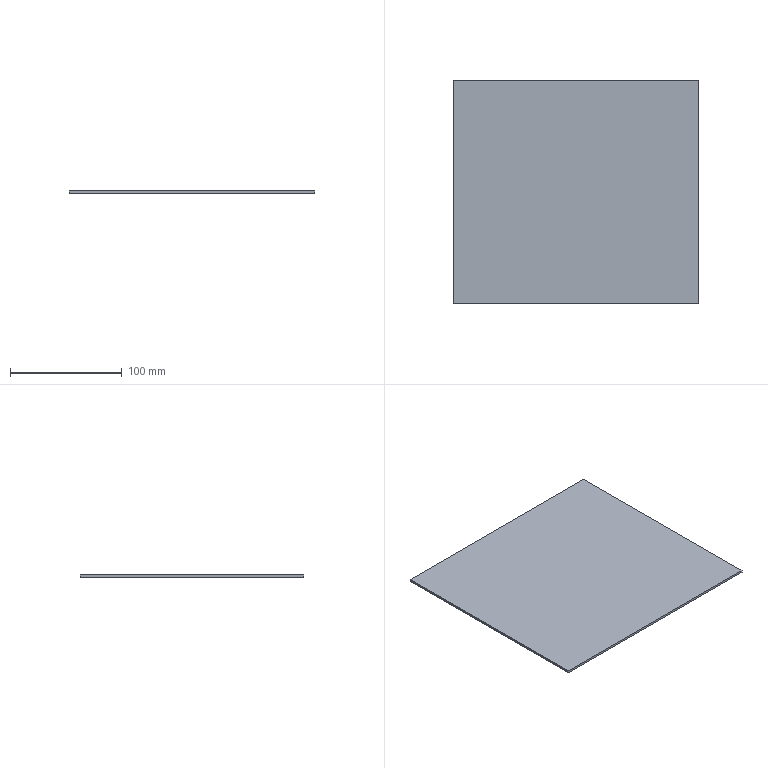Part | SolidWorks | features Extrusion 1 | 1 solid | 6 faces | box 220 x 200 x 2 mm | volume 88000 mm3 | plane 6
STEP:
#1=CARTESIAN_POINT('',(96.32,-91.,0.));
#2=VERTEX_POINT('',#1);
#3=CARTESIAN_POINT('',(96.32,109.,0.));
#4=VERTEX_POINT('',#3);
#5=CARTESIAN_POINT('',(96.32,-91.,0.));
#6=DIRECTION('',(0.,1.,0.));
#7=VECTOR('',#6,1000.);
#8=LINE('',#5,#7);
#9=EDGE_CURVE('',#2,#4,#8,.T.);
#10=ORIENTED_EDGE('',*,*,#9,.T.);
#11=CARTESIAN_POINT('',(96.32,109.,2.));
#12=VERTEX_POINT('',#11);
#13=CARTESIAN_POINT('',(96.32,109.,2.));
#14=DIRECTION('',(0.,0.,-1.));
#15=VECTOR('',#14,1000.);
#16=LINE('',#13,#15);
#17=EDGE_CURVE('',#12,#4,#16,.T.);
#18=ORIENTED_EDGE('',*,*,#17,.F.);
#19=CARTESIAN_POINT('',(96.32,-91.,2.));
#20=VERTEX_POINT('',#19);
#21=CARTESIAN_POINT('',(96.32,-91.,2.));
#22=DIRECTION('',(0.,1.,0.));
#23=VECTOR('',#22,1000.);
#24=LINE('',#21,#23);
#25=EDGE_CURVE('',#20,#12,#24,.T.);
#26=ORIENTED_EDGE('',*,*,#25,.F.);
#27=CARTESIAN_POINT('',(96.32,-91.,2.));
#28=DIRECTION('',(0.,0.,-1.));
#29=VECTOR('',#28,1000.);
#30=LINE('',#27,#29);
#31=EDGE_CURVE('',#20,#2,#30,.T.);
#32=ORIENTED_EDGE('',*,*,#31,.T.);
#33=EDGE_LOOP('',(#10,#18,#26,#32));
#34=FACE_OUTER_BOUND('',#33,.T.);
#35=CARTESIAN_POINT('',(96.32,-91.,2.));
#36=DIRECTION('',(-1.,0.,0.));
#37=DIRECTION('',(0.,0.,1.));
#38=AXIS2_PLACEMENT_3D('',#35,#36,#37);
#39=PLANE('',#38);
#40=ADVANCED_FACE('',(#34),#39,.F.);
#41=CARTESIAN_POINT('',(-123.68,109.,0.));
#42=VERTEX_POINT('',#41);
#43=CARTESIAN_POINT('',(96.32,109.,0.));
#44=DIRECTION('',(-1.,0.,0.));
#45=VECTOR('',#44,1000.);
#46=LINE('',#43,#45);
#47=EDGE_CURVE('',#4,#42,#46,.T.);
#48=ORIENTED_EDGE('',*,*,#47,.T.);
#49=CARTESIAN_POINT('',(-123.68,109.,2.));
#50=VERTEX_POINT('',#49);
#51=CARTESIAN_POINT('',(-123.68,109.,2.));
#52=DIRECTION('',(0.,0.,-1.));
#53=VECTOR('',#52,1000.);
#54=LINE('',#51,#53);
#55=EDGE_CURVE('',#50,#42,#54,.T.);
#56=ORIENTED_EDGE('',*,*,#55,.F.);
#57=CARTESIAN_POINT('',(96.32,109.,2.));
#58=DIRECTION('',(-1.,0.,0.));
#59=VECTOR('',#58,1000.);
#60=LINE('',#57,#59);
#61=EDGE_CURVE('',#12,#50,#60,.T.);
#62=ORIENTED_EDGE('',*,*,#61,.F.);
#63=ORIENTED_EDGE('',*,*,#17,.T.);
#64=EDGE_LOOP('',(#48,#56,#62,#63));
#65=FACE_OUTER_BOUND('',#64,.T.);
#66=CARTESIAN_POINT('',(96.32,109.,2.));
#67=DIRECTION('',(0.,-1.,0.));
#68=DIRECTION('',(1.,0.,0.));
#69=AXIS2_PLACEMENT_3D('',#66,#67,#68);
#70=PLANE('',#69);
#71=ADVANCED_FACE('',(#65),#70,.F.);
#72=CARTESIAN_POINT('',(-123.68,-91.,0.));
#73=VERTEX_POINT('',#72);
#74=CARTESIAN_POINT('',(-123.68,-91.,0.));
#75=DIRECTION('',(0.,1.,0.));
#76=VECTOR('',#75,1000.);
#77=LINE('',#74,#76);
#78=EDGE_CURVE('',#73,#42,#77,.T.);
#79=ORIENTED_EDGE('',*,*,#78,.F.);
#80=CARTESIAN_POINT('',(-123.68,-91.,2.));
#81=VERTEX_POINT('',#80);
#82=CARTESIAN_POINT('',(-123.68,-91.,2.));
#83=DIRECTION('',(0.,0.,-1.));
#84=VECTOR('',#83,1000.);
#85=LINE('',#82,#84);
#86=EDGE_CURVE('',#81,#73,#85,.T.);
#87=ORIENTED_EDGE('',*,*,#86,.F.);
#88=CARTESIAN_POINT('',(-123.68,-91.,2.));
#89=DIRECTION('',(0.,1.,0.));
#90=VECTOR('',#89,1000.);
#91=LINE('',#88,#90);
#92=EDGE_CURVE('',#81,#50,#91,.T.);
#93=ORIENTED_EDGE('',*,*,#92,.T.);
#94=ORIENTED_EDGE('',*,*,#55,.T.);
#95=EDGE_LOOP('',(#79,#87,#93,#94));
#96=FACE_OUTER_BOUND('',#95,.T.);
#97=CARTESIAN_POINT('',(-123.68,-91.,2.));
#98=DIRECTION('',(-1.,0.,0.));
#99=DIRECTION('',(0.,0.,1.));
#100=AXIS2_PLACEMENT_3D('',#97,#98,#99);
#101=PLANE('',#100);
#102=ADVANCED_FACE('',(#96),#101,.T.);
#103=CARTESIAN_POINT('',(96.32,-91.,0.));
#104=DIRECTION('',(-1.,0.,0.));
#105=VECTOR('',#104,1000.);
#106=LINE('',#103,#105);
#107=EDGE_CURVE('',#2,#73,#106,.T.);
#108=ORIENTED_EDGE('',*,*,#107,.F.);
#109=ORIENTED_EDGE('',*,*,#31,.F.);
#110=CARTESIAN_POINT('',(96.32,-91.,2.));
#111=DIRECTION('',(-1.,0.,0.));
#112=VECTOR('',#111,1000.);
#113=LINE('',#110,#112);
#114=EDGE_CURVE('',#20,#81,#113,.T.);
#115=ORIENTED_EDGE('',*,*,#114,.T.);
#116=ORIENTED_EDGE('',*,*,#86,.T.);
#117=EDGE_LOOP('',(#108,#109,#115,#116));
#118=FACE_OUTER_BOUND('',#117,.T.);
#119=CARTESIAN_POINT('',(96.32,-91.,2.));
#120=DIRECTION('',(0.,-1.,0.));
#121=DIRECTION('',(1.,0.,0.));
#122=AXIS2_PLACEMENT_3D('',#119,#120,#121);
#123=PLANE('',#122);
#124=ADVANCED_FACE('',(#118),#123,.T.);
#125=ORIENTED_EDGE('',*,*,#25,.T.);
#126=ORIENTED_EDGE('',*,*,#61,.T.);
#127=ORIENTED_EDGE('',*,*,#92,.F.);
#128=ORIENTED_EDGE('',*,*,#114,.F.);
#129=EDGE_LOOP('',(#125,#126,#127,#128));
#130=FACE_OUTER_BOUND('',#129,.T.);
#131=CARTESIAN_POINT('',(0.,0.,2.));
#132=DIRECTION('',(0.,0.,1.));
#133=DIRECTION('',(1.,0.,0.));
#134=AXIS2_PLACEMENT_3D('',#131,#132,#133);
#135=PLANE('',#134);
#136=ADVANCED_FACE('',(#130),#135,.T.);
#137=ORIENTED_EDGE('',*,*,#9,.F.);
#138=ORIENTED_EDGE('',*,*,#107,.T.);
#139=ORIENTED_EDGE('',*,*,#78,.T.);
#140=ORIENTED_EDGE('',*,*,#47,.F.);
#141=EDGE_LOOP('',(#137,#138,#139,#140));
#142=FACE_OUTER_BOUND('',#141,.T.);
#143=CARTESIAN_POINT('',(0.,0.,0.));
#144=DIRECTION('',(0.,0.,1.));
#145=DIRECTION('',(1.,0.,0.));
#146=AXIS2_PLACEMENT_3D('',#143,#144,#145);
#147=PLANE('',#146);
#148=ADVANCED_FACE('',(#142),#147,.F.);
#149=CLOSED_SHELL('',(#40,#71,#102,#124,#136,#148));
#150=MANIFOLD_SOLID_BREP('',#149);
#151=CARTESIAN_POINT('',(0.,0.,0.));
#152=DIRECTION('',(0.,0.,1.));
#153=DIRECTION('',(1.,0.,0.));
#154=AXIS2_PLACEMENT_3D('',#151,#152,#153);
#155=(LENGTH_UNIT()NAMED_UNIT(*)SI_UNIT(.MILLI.,.METRE.));
#156=UNCERTAINTY_MEASURE_WITH_UNIT(LENGTH_MEASURE(0.00001),#155,'','');
#157=(NAMED_UNIT(*)PLANE_ANGLE_UNIT()SI_UNIT($,.RADIAN.));
#158=(NAMED_UNIT(*)SI_UNIT($,.STERADIAN.)SOLID_ANGLE_UNIT());
#159=(GEOMETRIC_REPRESENTATION_CONTEXT(3)GLOBAL_UNCERTAINTY_ASSIGNED_CONTEXT((#156))GLOBAL_UNIT_ASSIGNED_CONTEXT((#155,#157,#158))REPRESENTATION_CONTEXT('',''));
#160=ADVANCED_BREP_SHAPE_REPRESENTATION('',(#150,#154),#159);